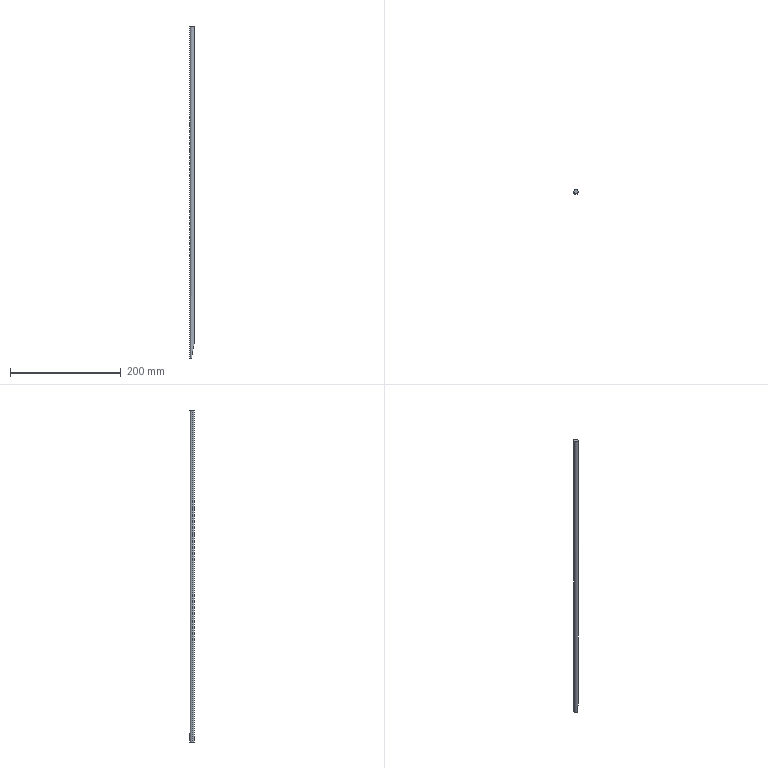Part | STEP file | 001-011-Blanking flip guide rod | 1 solid | 5 faces | box 8 x 8 x 600 mm | volume 29752 mm3 | plane 3 | cylinder 2 | commonest cylinder face diameters 8 x2
STEP:
#1=CARTESIAN_POINT('',(0.,0.,0.));
#2=DIRECTION('',(0.,0.,1.));
#3=DIRECTION('',(1.,0.,0.));
#4=AXIS2_PLACEMENT_3D('',#1,#2,#3);
#5=CARTESIAN_POINT('',(4.,0.,600.));
#6=VERTEX_POINT('',#5);
#7=CARTESIAN_POINT('',(-4.,0.,600.));
#8=VERTEX_POINT('',#7);
#9=CARTESIAN_POINT('',(0.,0.,600.));
#10=DIRECTION('',(0.,0.,1.));
#11=DIRECTION('',(1.,0.,0.));
#12=AXIS2_PLACEMENT_3D('',#9,#10,#11);
#13=CIRCLE('',#12,4.);
#14=CARTESIAN_POINT('',(0.,0.,600.));
#15=DIRECTION('',(0.,0.,-1.));
#16=DIRECTION('',(-1.,0.,0.));
#17=AXIS2_PLACEMENT_3D('',#14,#15,#16);
#18=CYLINDRICAL_SURFACE('',#17,4.);
#19=CARTESIAN_POINT('',(3.142,0.));
#20=DIRECTION('',(-1.,0.));
#21=VECTOR('',#20,1.);
#22=LINE('',#19,#21);
#23=(GEOMETRIC_REPRESENTATION_CONTEXT(2)PARAMETRIC_REPRESENTATION_CONTEXT()REPRESENTATION_CONTEXT('',''));
#24=DEFINITIONAL_REPRESENTATION('',(#22),#23);
#25=PCURVE('',#18,#24);
#26=CARTESIAN_POINT('',(0.,0.,600.));
#27=DIRECTION('',(0.,0.,1.));
#28=DIRECTION('',(1.,0.,0.));
#29=AXIS2_PLACEMENT_3D('',#26,#27,#28);
#30=PLANE('',#29);
#31=CARTESIAN_POINT('',(0.,0.));
#32=DIRECTION('',(1.,0.));
#33=AXIS2_PLACEMENT_2D('',#31,#32);
#34=CIRCLE('',#33,4.);
#35=(GEOMETRIC_REPRESENTATION_CONTEXT(2)PARAMETRIC_REPRESENTATION_CONTEXT()REPRESENTATION_CONTEXT('',''));
#36=DEFINITIONAL_REPRESENTATION('',(#34),#35);
#37=PCURVE('',#30,#36);
#38=SURFACE_CURVE('',#13,(#25,#37),.PCURVE_S1.);
#39=EDGE_CURVE('',#6,#8,#38,.T.);
#40=ORIENTED_EDGE('',*,*,#39,.F.);
#41=CARTESIAN_POINT('',(4.,0.,28.356));
#42=VERTEX_POINT('',#41);
#43=CARTESIAN_POINT('',(4.,0.,600.));
#44=DIRECTION('',(0.,0.,-1.));
#45=VECTOR('',#44,1.);
#46=LINE('',#43,#45);
#47=CARTESIAN_POINT('',(3.142,0.));
#48=DIRECTION('',(0.,1.));
#49=VECTOR('',#48,1.);
#50=LINE('',#47,#49);
#51=(GEOMETRIC_REPRESENTATION_CONTEXT(2)PARAMETRIC_REPRESENTATION_CONTEXT()REPRESENTATION_CONTEXT('',''));
#52=DEFINITIONAL_REPRESENTATION('',(#50),#51);
#53=PCURVE('',#18,#52);
#54=CARTESIAN_POINT('',(0.,0.,600.));
#55=DIRECTION('',(0.,0.,-1.));
#56=DIRECTION('',(-1.,0.,0.));
#57=AXIS2_PLACEMENT_3D('',#54,#55,#56);
#58=CYLINDRICAL_SURFACE('',#57,4.);
#59=CARTESIAN_POINT('',(3.142,0.));
#60=DIRECTION('',(0.,1.));
#61=VECTOR('',#60,1.);
#62=LINE('',#59,#61);
#63=(GEOMETRIC_REPRESENTATION_CONTEXT(2)PARAMETRIC_REPRESENTATION_CONTEXT()REPRESENTATION_CONTEXT('',''));
#64=DEFINITIONAL_REPRESENTATION('',(#62),#63);
#65=PCURVE('',#58,#64);
#66=SURFACE_CURVE('',#46,(#53,#65),.PCURVE_S1.);
#67=EDGE_CURVE('',#6,#42,#66,.T.);
#68=ORIENTED_EDGE('',*,*,#67,.T.);
#69=CARTESIAN_POINT('',(-1.,3.873,0.));
#70=VERTEX_POINT('',#69);
#71=CARTESIAN_POINT('',(4.,0.,28.356));
#72=CARTESIAN_POINT('',(4.,2.843,28.356));
#73=CARTESIAN_POINT('',(1.753,4.584,15.61));
#74=CARTESIAN_POINT('',(-1.,3.873,0.));
#75=(BOUNDED_CURVE()B_SPLINE_CURVE(3,(#71,#72,#73,#74),.UNSPECIFIED.,.F.,.F.)B_SPLINE_CURVE_WITH_KNOTS((4,4),(3.142,4.965),.PIECEWISE_BEZIER_KNOTS.)CURVE()GEOMETRIC_REPRESENTATION_ITEM()RATIONAL_B_SPLINE_CURVE((1.,0.7416,0.7416,1.))REPRESENTATION_ITEM(''));
#76=CARTESIAN_POINT('',(3.142,571.644));
#77=CARTESIAN_POINT('',(3.118,571.643));
#78=CARTESIAN_POINT('',(3.069,571.683));
#79=CARTESIAN_POINT('',(2.993,571.871));
#80=CARTESIAN_POINT('',(2.915,572.199));
#81=CARTESIAN_POINT('',(2.835,572.677));
#82=CARTESIAN_POINT('',(2.753,573.312));
#83=CARTESIAN_POINT('',(2.669,574.109));
#84=CARTESIAN_POINT('',(2.583,575.068));
#85=CARTESIAN_POINT('',(2.496,576.187));
#86=CARTESIAN_POINT('',(2.408,577.46));
#87=CARTESIAN_POINT('',(2.319,578.875));
#88=CARTESIAN_POINT('',(2.23,580.419));
#89=CARTESIAN_POINT('',(2.141,582.073));
#90=CARTESIAN_POINT('',(2.052,583.817));
#91=CARTESIAN_POINT('',(1.964,585.63));
#92=CARTESIAN_POINT('',(1.877,587.487));
#93=CARTESIAN_POINT('',(1.791,589.367));
#94=CARTESIAN_POINT('',(1.707,591.247));
#95=CARTESIAN_POINT('',(1.625,593.107));
#96=CARTESIAN_POINT('',(1.544,594.928));
#97=CARTESIAN_POINT('',(1.466,596.694));
#98=CARTESIAN_POINT('',(1.391,598.393));
#99=CARTESIAN_POINT('',(1.342,599.474));
#100=CARTESIAN_POINT('',(1.318,600.));
#101=B_SPLINE_CURVE_WITH_KNOTS('',3,(#76,#77,#78,#79,#80,#81,#82,#83,#84,#85,#86,#87,#88,#89,#90,#91,#92,#93,#94,#95,#96,#97,#98,#99,#100),.UNSPECIFIED.,.F.,.F.,(4,1,1,1,1,1,1,1,1,1,1,1,1,1,1,1,1,1,1,1,1,1,4),(3.142,3.224,3.307,3.39,3.473,3.556,3.639,3.722,3.805,3.888,3.97,4.053,4.136,4.219,4.302,4.385,4.468,4.551,4.634,4.716,4.799,4.882,4.965),.QUASI_UNIFORM_KNOTS.);
#102=(GEOMETRIC_REPRESENTATION_CONTEXT(2)PARAMETRIC_REPRESENTATION_CONTEXT()REPRESENTATION_CONTEXT('',''));
#103=DEFINITIONAL_REPRESENTATION('',(#101),#102);
#104=PCURVE('',#18,#103);
#105=CARTESIAN_POINT('',(-1.,-4.,0.));
#106=DIRECTION('',(-0.9848,0.,0.1736));
#107=DIRECTION('',(0.1736,0.,0.9848));
#108=AXIS2_PLACEMENT_3D('',#105,#106,#107);
#109=PLANE('',#108);
#110=CARTESIAN_POINT('',(28.794,4.));
#111=CARTESIAN_POINT('',(28.794,6.843));
#112=CARTESIAN_POINT('',(15.851,8.584));
#113=CARTESIAN_POINT('',(0.,7.873));
#114=(BOUNDED_CURVE()B_SPLINE_CURVE(3,(#110,#111,#112,#113),.UNSPECIFIED.,.F.,.F.)B_SPLINE_CURVE_WITH_KNOTS((4,4),(3.142,4.965),.PIECEWISE_BEZIER_KNOTS.)CURVE()GEOMETRIC_REPRESENTATION_ITEM()RATIONAL_B_SPLINE_CURVE((1.,0.7416,0.7416,1.))REPRESENTATION_ITEM(''));
#115=(GEOMETRIC_REPRESENTATION_CONTEXT(2)PARAMETRIC_REPRESENTATION_CONTEXT()REPRESENTATION_CONTEXT('',''));
#116=DEFINITIONAL_REPRESENTATION('',(#114),#115);
#117=PCURVE('',#109,#116);
#118=SURFACE_CURVE('',#75,(#104,#117),.PCURVE_S1.);
#119=EDGE_CURVE('',#42,#70,#118,.T.);
#120=ORIENTED_EDGE('',*,*,#119,.T.);
#121=CARTESIAN_POINT('',(-4.,0.,0.));
#122=VERTEX_POINT('',#121);
#123=CARTESIAN_POINT('',(0.,0.,0.));
#124=DIRECTION('',(0.,0.,1.));
#125=DIRECTION('',(1.,0.,0.));
#126=AXIS2_PLACEMENT_3D('',#123,#124,#125);
#127=CIRCLE('',#126,4.);
#128=CARTESIAN_POINT('',(3.142,600.));
#129=DIRECTION('',(-1.,0.));
#130=VECTOR('',#129,1.);
#131=LINE('',#128,#130);
#132=(GEOMETRIC_REPRESENTATION_CONTEXT(2)PARAMETRIC_REPRESENTATION_CONTEXT()REPRESENTATION_CONTEXT('',''));
#133=DEFINITIONAL_REPRESENTATION('',(#131),#132);
#134=PCURVE('',#18,#133);
#135=CARTESIAN_POINT('',(0.,0.,0.));
#136=DIRECTION('',(0.,0.,1.));
#137=DIRECTION('',(1.,0.,0.));
#138=AXIS2_PLACEMENT_3D('',#135,#136,#137);
#139=PLANE('',#138);
#140=CARTESIAN_POINT('',(0.,0.));
#141=DIRECTION('',(1.,0.));
#142=AXIS2_PLACEMENT_2D('',#140,#141);
#143=CIRCLE('',#142,4.);
#144=(GEOMETRIC_REPRESENTATION_CONTEXT(2)PARAMETRIC_REPRESENTATION_CONTEXT()REPRESENTATION_CONTEXT('',''));
#145=DEFINITIONAL_REPRESENTATION('',(#143),#144);
#146=PCURVE('',#139,#145);
#147=SURFACE_CURVE('',#127,(#134,#146),.PCURVE_S1.);
#148=EDGE_CURVE('',#70,#122,#147,.T.);
#149=ORIENTED_EDGE('',*,*,#148,.T.);
#150=CARTESIAN_POINT('',(-4.,0.,600.));
#151=DIRECTION('',(0.,0.,-1.));
#152=VECTOR('',#151,1.);
#153=LINE('',#150,#152);
#154=CARTESIAN_POINT('',(0.,0.));
#155=DIRECTION('',(0.,1.));
#156=VECTOR('',#155,1.);
#157=LINE('',#154,#156);
#158=(GEOMETRIC_REPRESENTATION_CONTEXT(2)PARAMETRIC_REPRESENTATION_CONTEXT()REPRESENTATION_CONTEXT('',''));
#159=DEFINITIONAL_REPRESENTATION('',(#157),#158);
#160=PCURVE('',#18,#159);
#161=CARTESIAN_POINT('',(6.283,0.));
#162=DIRECTION('',(0.,1.));
#163=VECTOR('',#162,1.);
#164=LINE('',#161,#163);
#165=(GEOMETRIC_REPRESENTATION_CONTEXT(2)PARAMETRIC_REPRESENTATION_CONTEXT()REPRESENTATION_CONTEXT('',''));
#166=DEFINITIONAL_REPRESENTATION('',(#164),#165);
#167=PCURVE('',#58,#166);
#168=SURFACE_CURVE('',#153,(#160,#167),.PCURVE_S1.);
#169=EDGE_CURVE('',#8,#122,#168,.T.);
#170=ORIENTED_EDGE('',*,*,#169,.F.);
#171=EDGE_LOOP('',(#40,#68,#120,#149,#170));
#172=FACE_BOUND('',#171,.T.);
#173=ADVANCED_FACE('',(#172),#18,.T.);
#174=ORIENTED_EDGE('',*,*,#67,.F.);
#175=CARTESIAN_POINT('',(0.,0.,600.));
#176=DIRECTION('',(0.,0.,1.));
#177=DIRECTION('',(1.,0.,0.));
#178=AXIS2_PLACEMENT_3D('',#175,#176,#177);
#179=CIRCLE('',#178,4.);
#180=CARTESIAN_POINT('',(9.425,0.));
#181=DIRECTION('',(-1.,0.));
#182=VECTOR('',#181,1.);
#183=LINE('',#180,#182);
#184=(GEOMETRIC_REPRESENTATION_CONTEXT(2)PARAMETRIC_REPRESENTATION_CONTEXT()REPRESENTATION_CONTEXT('',''));
#185=DEFINITIONAL_REPRESENTATION('',(#183),#184);
#186=PCURVE('',#58,#185);
#187=CARTESIAN_POINT('',(0.,0.));
#188=DIRECTION('',(1.,0.));
#189=AXIS2_PLACEMENT_2D('',#187,#188);
#190=CIRCLE('',#189,4.);
#191=(GEOMETRIC_REPRESENTATION_CONTEXT(2)PARAMETRIC_REPRESENTATION_CONTEXT()REPRESENTATION_CONTEXT('',''));
#192=DEFINITIONAL_REPRESENTATION('',(#190),#191);
#193=PCURVE('',#30,#192);
#194=SURFACE_CURVE('',#179,(#186,#193),.PCURVE_S1.);
#195=EDGE_CURVE('',#8,#6,#194,.T.);
#196=ORIENTED_EDGE('',*,*,#195,.F.);
#197=ORIENTED_EDGE('',*,*,#169,.T.);
#198=CARTESIAN_POINT('',(-1.,-3.873,0.));
#199=VERTEX_POINT('',#198);
#200=CARTESIAN_POINT('',(0.,0.,0.));
#201=DIRECTION('',(0.,0.,1.));
#202=DIRECTION('',(1.,0.,0.));
#203=AXIS2_PLACEMENT_3D('',#200,#201,#202);
#204=CIRCLE('',#203,4.);
#205=CARTESIAN_POINT('',(9.425,600.));
#206=DIRECTION('',(-1.,0.));
#207=VECTOR('',#206,1.);
#208=LINE('',#205,#207);
#209=(GEOMETRIC_REPRESENTATION_CONTEXT(2)PARAMETRIC_REPRESENTATION_CONTEXT()REPRESENTATION_CONTEXT('',''));
#210=DEFINITIONAL_REPRESENTATION('',(#208),#209);
#211=PCURVE('',#58,#210);
#212=CARTESIAN_POINT('',(0.,0.));
#213=DIRECTION('',(1.,0.));
#214=AXIS2_PLACEMENT_2D('',#212,#213);
#215=CIRCLE('',#214,4.);
#216=(GEOMETRIC_REPRESENTATION_CONTEXT(2)PARAMETRIC_REPRESENTATION_CONTEXT()REPRESENTATION_CONTEXT('',''));
#217=DEFINITIONAL_REPRESENTATION('',(#215),#216);
#218=PCURVE('',#139,#217);
#219=SURFACE_CURVE('',#204,(#211,#218),.PCURVE_S1.);
#220=EDGE_CURVE('',#122,#199,#219,.T.);
#221=ORIENTED_EDGE('',*,*,#220,.T.);
#222=CARTESIAN_POINT('',(-1.,-3.873,0.));
#223=CARTESIAN_POINT('',(1.753,-4.584,15.61));
#224=CARTESIAN_POINT('',(4.,-2.843,28.356));
#225=CARTESIAN_POINT('',(4.,0.,28.356));
#226=(BOUNDED_CURVE()B_SPLINE_CURVE(3,(#222,#223,#224,#225),.UNSPECIFIED.,.F.,.F.)B_SPLINE_CURVE_WITH_KNOTS((4,4),(1.318,3.142),.PIECEWISE_BEZIER_KNOTS.)CURVE()GEOMETRIC_REPRESENTATION_ITEM()RATIONAL_B_SPLINE_CURVE((1.,0.7416,0.7416,1.))REPRESENTATION_ITEM(''));
#227=CARTESIAN_POINT('',(4.965,600.));
#228=CARTESIAN_POINT('',(4.941,599.474));
#229=CARTESIAN_POINT('',(4.892,598.393));
#230=CARTESIAN_POINT('',(4.817,596.694));
#231=CARTESIAN_POINT('',(4.739,594.928));
#232=CARTESIAN_POINT('',(4.659,593.107));
#233=CARTESIAN_POINT('',(4.576,591.247));
#234=CARTESIAN_POINT('',(4.492,589.367));
#235=CARTESIAN_POINT('',(4.406,587.487));
#236=CARTESIAN_POINT('',(4.319,585.63));
#237=CARTESIAN_POINT('',(4.231,583.817));
#238=CARTESIAN_POINT('',(4.142,582.073));
#239=CARTESIAN_POINT('',(4.053,580.419));
#240=CARTESIAN_POINT('',(3.964,578.875));
#241=CARTESIAN_POINT('',(3.875,577.46));
#242=CARTESIAN_POINT('',(3.787,576.187));
#243=CARTESIAN_POINT('',(3.7,575.068));
#244=CARTESIAN_POINT('',(3.614,574.109));
#245=CARTESIAN_POINT('',(3.53,573.312));
#246=CARTESIAN_POINT('',(3.448,572.677));
#247=CARTESIAN_POINT('',(3.368,572.199));
#248=CARTESIAN_POINT('',(3.29,571.871));
#249=CARTESIAN_POINT('',(3.214,571.683));
#250=CARTESIAN_POINT('',(3.166,571.643));
#251=CARTESIAN_POINT('',(3.142,571.644));
#252=B_SPLINE_CURVE_WITH_KNOTS('',3,(#227,#228,#229,#230,#231,#232,#233,#234,#235,#236,#237,#238,#239,#240,#241,#242,#243,#244,#245,#246,#247,#248,#249,#250,#251),.UNSPECIFIED.,.F.,.F.,(4,1,1,1,1,1,1,1,1,1,1,1,1,1,1,1,1,1,1,1,1,1,4),(1.318,1.401,1.484,1.567,1.65,1.733,1.815,1.898,1.981,2.064,2.147,2.23,2.313,2.396,2.479,2.561,2.644,2.727,2.81,2.893,2.976,3.059,3.142),.QUASI_UNIFORM_KNOTS.);
#253=(GEOMETRIC_REPRESENTATION_CONTEXT(2)PARAMETRIC_REPRESENTATION_CONTEXT()REPRESENTATION_CONTEXT('',''));
#254=DEFINITIONAL_REPRESENTATION('',(#252),#253);
#255=PCURVE('',#58,#254);
#256=CARTESIAN_POINT('',(0.,0.127));
#257=CARTESIAN_POINT('',(15.851,-0.5837));
#258=CARTESIAN_POINT('',(28.794,1.157));
#259=CARTESIAN_POINT('',(28.794,4.));
#260=(BOUNDED_CURVE()B_SPLINE_CURVE(3,(#256,#257,#258,#259),.UNSPECIFIED.,.F.,.F.)B_SPLINE_CURVE_WITH_KNOTS((4,4),(1.318,3.142),.PIECEWISE_BEZIER_KNOTS.)CURVE()GEOMETRIC_REPRESENTATION_ITEM()RATIONAL_B_SPLINE_CURVE((1.,0.7416,0.7416,1.))REPRESENTATION_ITEM(''));
#261=(GEOMETRIC_REPRESENTATION_CONTEXT(2)PARAMETRIC_REPRESENTATION_CONTEXT()REPRESENTATION_CONTEXT('',''));
#262=DEFINITIONAL_REPRESENTATION('',(#260),#261);
#263=PCURVE('',#109,#262);
#264=SURFACE_CURVE('',#226,(#255,#263),.PCURVE_S1.);
#265=EDGE_CURVE('',#199,#42,#264,.T.);
#266=ORIENTED_EDGE('',*,*,#265,.T.);
#267=EDGE_LOOP('',(#174,#196,#197,#221,#266));
#268=FACE_BOUND('',#267,.T.);
#269=ADVANCED_FACE('',(#268),#58,.T.);
#270=ORIENTED_EDGE('',*,*,#195,.T.);
#271=ORIENTED_EDGE('',*,*,#39,.T.);
#272=EDGE_LOOP('',(#270,#271));
#273=FACE_BOUND('',#272,.T.);
#274=ADVANCED_FACE('',(#273),#30,.T.);
#275=ORIENTED_EDGE('',*,*,#148,.F.);
#276=CARTESIAN_POINT('',(-1.,0.,0.));
#277=DIRECTION('',(0.,-1.,0.));
#278=VECTOR('',#277,1.);
#279=LINE('',#276,#278);
#280=CARTESIAN_POINT('',(-1.,0.));
#281=DIRECTION('',(0.,-1.));
#282=VECTOR('',#281,1.);
#283=LINE('',#280,#282);
#284=(GEOMETRIC_REPRESENTATION_CONTEXT(2)PARAMETRIC_REPRESENTATION_CONTEXT()REPRESENTATION_CONTEXT('',''));
#285=DEFINITIONAL_REPRESENTATION('',(#283),#284);
#286=PCURVE('',#139,#285);
#287=CARTESIAN_POINT('',(0.,4.));
#288=DIRECTION('',(0.,-1.));
#289=VECTOR('',#288,1.);
#290=LINE('',#287,#289);
#291=(GEOMETRIC_REPRESENTATION_CONTEXT(2)PARAMETRIC_REPRESENTATION_CONTEXT()REPRESENTATION_CONTEXT('',''));
#292=DEFINITIONAL_REPRESENTATION('',(#290),#291);
#293=PCURVE('',#109,#292);
#294=SURFACE_CURVE('',#279,(#286,#293),.PCURVE_S1.);
#295=EDGE_CURVE('',#70,#199,#294,.T.);
#296=ORIENTED_EDGE('',*,*,#295,.T.);
#297=ORIENTED_EDGE('',*,*,#220,.F.);
#298=EDGE_LOOP('',(#275,#296,#297));
#299=FACE_BOUND('',#298,.T.);
#300=ADVANCED_FACE('',(#299),#139,.F.);
#301=ORIENTED_EDGE('',*,*,#295,.F.);
#302=ORIENTED_EDGE('',*,*,#119,.F.);
#303=ORIENTED_EDGE('',*,*,#265,.F.);
#304=EDGE_LOOP('',(#301,#302,#303));
#305=FACE_BOUND('',#304,.T.);
#306=ADVANCED_FACE('',(#305),#109,.F.);
#307=CLOSED_SHELL('',(#173,#269,#274,#300,#306));
#308=MANIFOLD_SOLID_BREP('',#307);
#309=(LENGTH_UNIT()NAMED_UNIT(*)SI_UNIT(.MILLI.,.METRE.));
#310=UNCERTAINTY_MEASURE_WITH_UNIT(LENGTH_MEASURE(0.0000001),#309,'','');
#311=(NAMED_UNIT(*)PLANE_ANGLE_UNIT()SI_UNIT($,.RADIAN.));
#312=(NAMED_UNIT(*)SI_UNIT($,.STERADIAN.)SOLID_ANGLE_UNIT());
#313=(GEOMETRIC_REPRESENTATION_CONTEXT(3)GLOBAL_UNCERTAINTY_ASSIGNED_CONTEXT((#310))GLOBAL_UNIT_ASSIGNED_CONTEXT((#309,#311,#312))REPRESENTATION_CONTEXT('',''));
#314=ADVANCED_BREP_SHAPE_REPRESENTATION('',(#4,#308),#313);